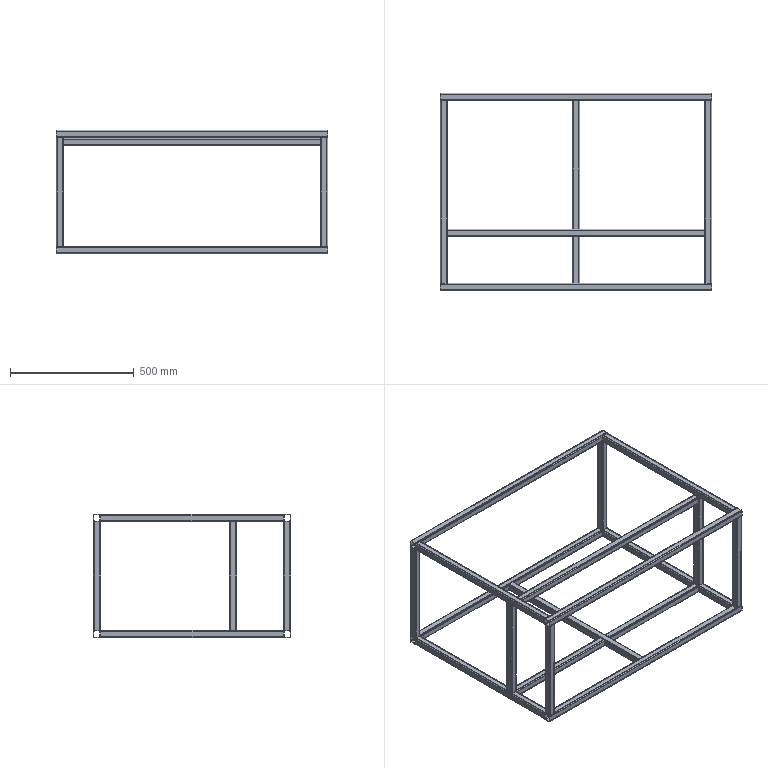Part | SolidWorks | features 3DProfileFeature 1, WeldMemberFeat 1, WeldmentFeature 1 | 18 solids | 324 faces | box 1098 x 797.6 x 498.8 mm | volume 3412994 mm3 | plane 180 | cylinder 144 | commonest cylinder face diameters 5.2 x72 10.4 x72